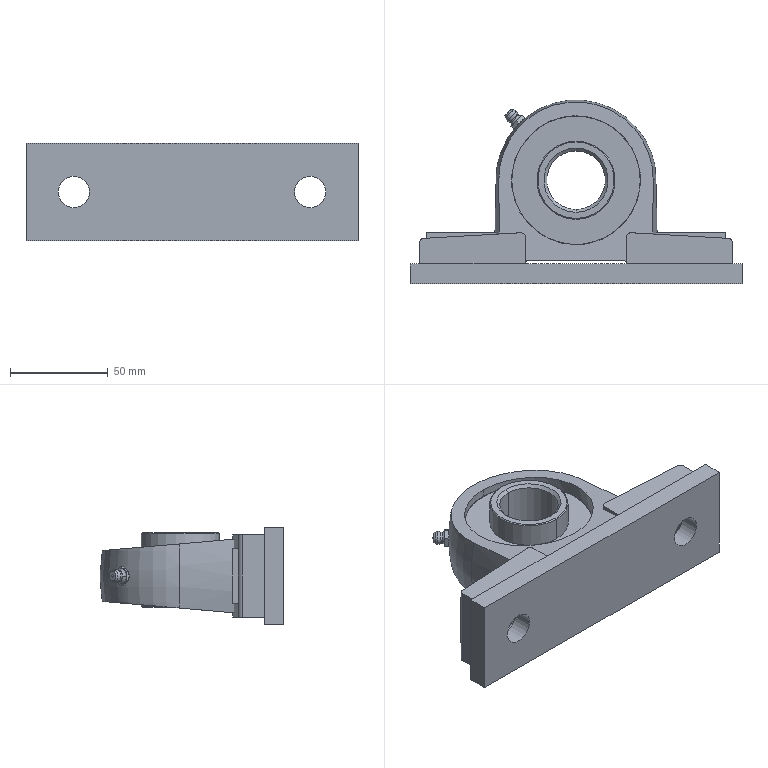Part | STEP file | ucp206 z blacha1V11 | 2 solids | 131 faces | box 170 x 94 x 50 mm | volume 262085 mm3 | plane 62 | cylinder 40 | cone 17 | torus 8 | sphere 3 | other 1 | commonest cylinder face diameters 4 x16 17 x6 16 x4 40.1 x4 66 x4 6 x2